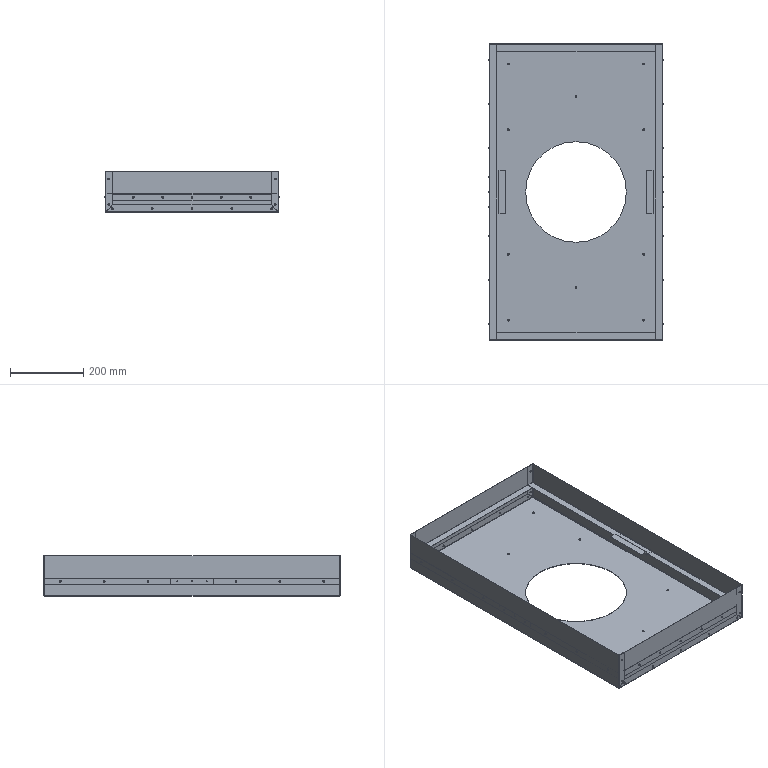Part | SolidWorks | features ReferencePattern 23, CompositeCurve 6, MirrorCompFeat 2 | 51 solids | 944 faces | box 477.6 x 813.6 x 111 mm | volume 709614 mm3 | cylinder 506 | plane 330 | sphere 84 | cone 16 | spline 8 | commonest cylinder face diameters 2.4 x180 2.5 x168 2.65 x84 5 x20 1.473 x18 3.2 x16